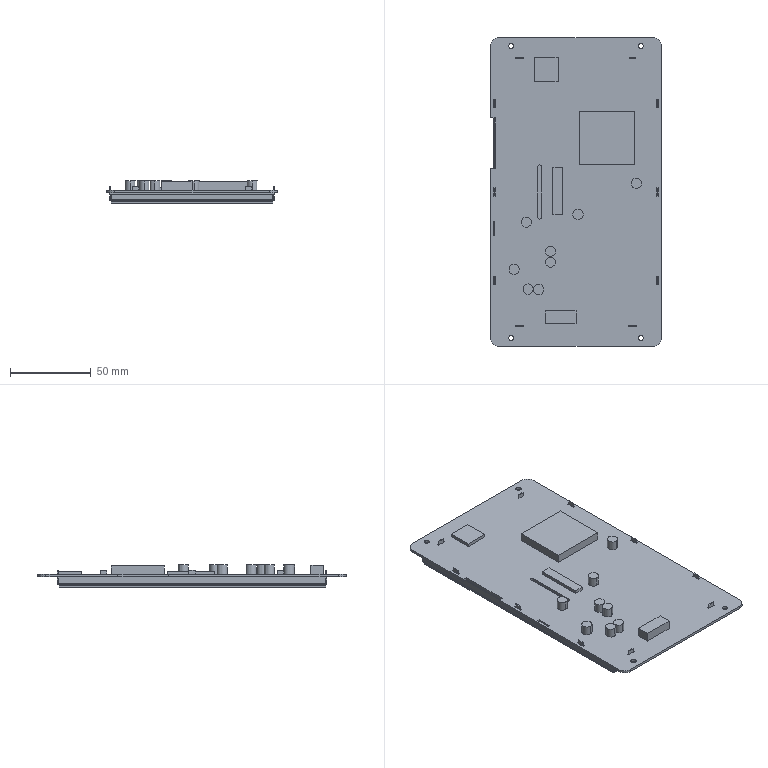Part | STEP file | DMG10600T070_01WTC_X2_8FEA658_2 | 1 solid | 253 faces | box 105.41 x 190.5 x 13.675 mm | volume 120263 mm3 | plane 223 | cylinder 30 | commonest cylinder face diameters 6.3 x16 3.2 x8 10.16 x4 2.032 x2